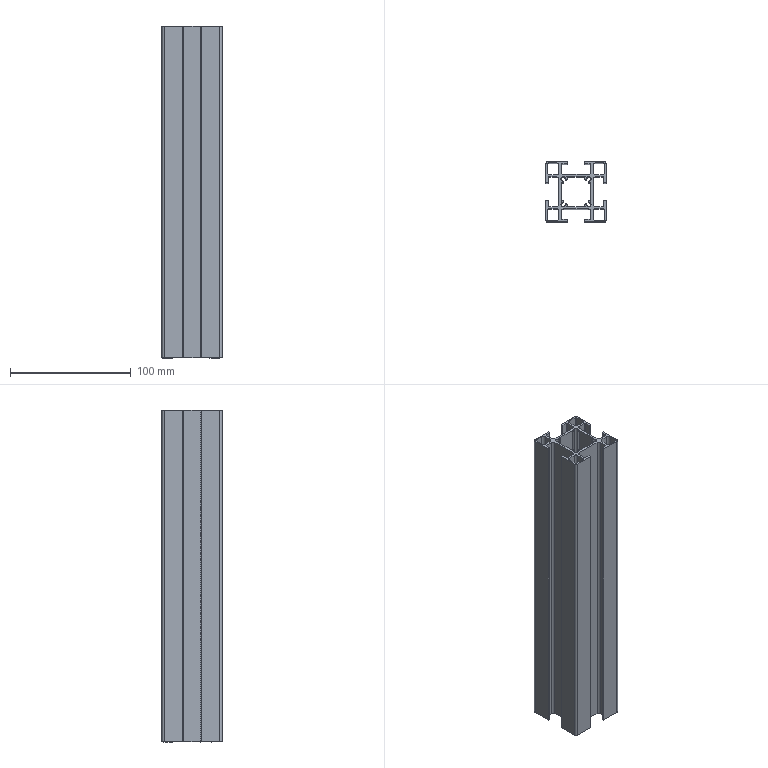Part | STEP file | 46A-00006CC11-275mm | 1 solid | 142 faces | box 50 x 50 x 275 mm | volume 161560 mm3 | cylinder 84 | plane 58 | commonest cylinder face diameters 1 x24 4 x24 1.5 x16 3.7 x8 6.7 x8 2 x4